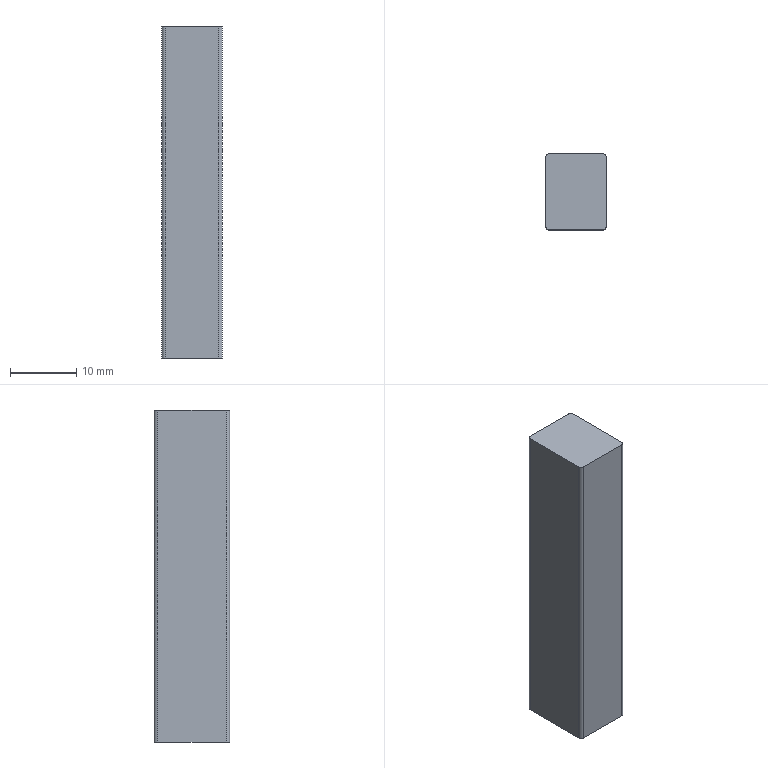Part | NX | features BREP 1 | 1 solid | 10 faces | box 9.124 x 11.391 x 50 mm | volume 5186 mm3 | plane 6 | cylinder 4 | commonest cylinder face diameters 1 x4
STEP:
#1=CARTESIAN_POINT('',(-4.062,5.695,-40.6));
#2=VERTEX_POINT('',#1);
#3=CARTESIAN_POINT('',(-4.562,5.195,-40.6));
#4=VERTEX_POINT('',#3);
#5=CARTESIAN_POINT('',(-4.062,5.195,-40.6));
#6=DIRECTION('',(0.,0.,1.));
#7=DIRECTION('',(1.,0.,0.));
#8=AXIS2_PLACEMENT_3D('',#5,#6,#7);
#9=CIRCLE('',#8,0.5);
#10=EDGE_CURVE('',#2,#4,#9,.T.);
#11=ORIENTED_EDGE('',*,*,#10,.F.);
#12=CARTESIAN_POINT('',(-4.062,5.695,-90.6));
#13=VERTEX_POINT('',#12);
#14=CARTESIAN_POINT('',(-4.062,5.695,-90.6));
#15=DIRECTION('',(0.,0.,1.));
#16=VECTOR('',#15,1000.);
#17=LINE('',#14,#16);
#18=EDGE_CURVE('',#13,#2,#17,.T.);
#19=ORIENTED_EDGE('',*,*,#18,.F.);
#20=CARTESIAN_POINT('',(-4.562,5.195,-90.6));
#21=VERTEX_POINT('',#20);
#22=CARTESIAN_POINT('',(-4.062,5.195,-90.6));
#23=DIRECTION('',(0.,0.,1.));
#24=DIRECTION('',(1.,0.,0.));
#25=AXIS2_PLACEMENT_3D('',#22,#23,#24);
#26=CIRCLE('',#25,0.5);
#27=EDGE_CURVE('',#13,#21,#26,.T.);
#28=ORIENTED_EDGE('',*,*,#27,.T.);
#29=CARTESIAN_POINT('',(-4.562,5.195,-90.6));
#30=DIRECTION('',(0.,0.,1.));
#31=VECTOR('',#30,1000.);
#32=LINE('',#29,#31);
#33=EDGE_CURVE('',#21,#4,#32,.T.);
#34=ORIENTED_EDGE('',*,*,#33,.T.);
#35=EDGE_LOOP('',(#11,#19,#28,#34));
#36=FACE_BOUND('',#35,.T.);
#37=CARTESIAN_POINT('',(-4.062,5.195,-90.6));
#38=DIRECTION('',(0.,0.,1.));
#39=DIRECTION('',(-1.,0.,0.));
#40=AXIS2_PLACEMENT_3D('',#37,#38,#39);
#41=CYLINDRICAL_SURFACE('',#40,0.5);
#42=ADVANCED_FACE('',(#36),#41,.T.);
#43=CARTESIAN_POINT('',(-4.562,-5.195,-40.6));
#44=VERTEX_POINT('',#43);
#45=CARTESIAN_POINT('',(-4.562,-5.195,-40.6));
#46=DIRECTION('',(0.,1.,0.));
#47=VECTOR('',#46,1000.);
#48=LINE('',#45,#47);
#49=EDGE_CURVE('',#44,#4,#48,.T.);
#50=ORIENTED_EDGE('',*,*,#49,.T.);
#51=ORIENTED_EDGE('',*,*,#33,.F.);
#52=CARTESIAN_POINT('',(-4.562,-5.195,-90.6));
#53=VERTEX_POINT('',#52);
#54=CARTESIAN_POINT('',(-4.562,-5.195,-90.6));
#55=DIRECTION('',(0.,1.,0.));
#56=VECTOR('',#55,1000.);
#57=LINE('',#54,#56);
#58=EDGE_CURVE('',#53,#21,#57,.T.);
#59=ORIENTED_EDGE('',*,*,#58,.F.);
#60=CARTESIAN_POINT('',(-4.562,-5.195,-90.6));
#61=DIRECTION('',(0.,0.,1.));
#62=VECTOR('',#61,1000.);
#63=LINE('',#60,#62);
#64=EDGE_CURVE('',#53,#44,#63,.T.);
#65=ORIENTED_EDGE('',*,*,#64,.T.);
#66=EDGE_LOOP('',(#50,#51,#59,#65));
#67=FACE_BOUND('',#66,.T.);
#68=CARTESIAN_POINT('',(-4.562,-5.195,-90.6));
#69=DIRECTION('',(1.,0.,0.));
#70=DIRECTION('',(0.,-1.,0.));
#71=AXIS2_PLACEMENT_3D('',#68,#69,#70);
#72=PLANE('',#71);
#73=ADVANCED_FACE('',(#67),#72,.F.);
#74=CARTESIAN_POINT('',(-4.062,-5.695,-40.6));
#75=VERTEX_POINT('',#74);
#76=CARTESIAN_POINT('',(-4.062,-5.195,-40.6));
#77=DIRECTION('',(0.,0.,1.));
#78=DIRECTION('',(1.,0.,0.));
#79=AXIS2_PLACEMENT_3D('',#76,#77,#78);
#80=CIRCLE('',#79,0.5);
#81=EDGE_CURVE('',#44,#75,#80,.T.);
#82=ORIENTED_EDGE('',*,*,#81,.F.);
#83=ORIENTED_EDGE('',*,*,#64,.F.);
#84=CARTESIAN_POINT('',(-4.062,-5.695,-90.6));
#85=VERTEX_POINT('',#84);
#86=CARTESIAN_POINT('',(-4.062,-5.195,-90.6));
#87=DIRECTION('',(0.,0.,1.));
#88=DIRECTION('',(1.,0.,0.));
#89=AXIS2_PLACEMENT_3D('',#86,#87,#88);
#90=CIRCLE('',#89,0.5);
#91=EDGE_CURVE('',#53,#85,#90,.T.);
#92=ORIENTED_EDGE('',*,*,#91,.T.);
#93=CARTESIAN_POINT('',(-4.062,-5.695,-90.6));
#94=DIRECTION('',(0.,0.,1.));
#95=VECTOR('',#94,1000.);
#96=LINE('',#93,#95);
#97=EDGE_CURVE('',#85,#75,#96,.T.);
#98=ORIENTED_EDGE('',*,*,#97,.T.);
#99=EDGE_LOOP('',(#82,#83,#92,#98));
#100=FACE_BOUND('',#99,.T.);
#101=CARTESIAN_POINT('',(-4.062,-5.195,-90.6));
#102=DIRECTION('',(0.,0.,1.));
#103=DIRECTION('',(-1.,0.,0.));
#104=AXIS2_PLACEMENT_3D('',#101,#102,#103);
#105=CYLINDRICAL_SURFACE('',#104,0.5);
#106=ADVANCED_FACE('',(#100),#105,.T.);
#107=CARTESIAN_POINT('',(4.062,-5.695,-40.6));
#108=VERTEX_POINT('',#107);
#109=CARTESIAN_POINT('',(4.062,-5.695,-40.6));
#110=DIRECTION('',(-1.,0.,0.));
#111=VECTOR('',#110,1000.);
#112=LINE('',#109,#111);
#113=EDGE_CURVE('',#108,#75,#112,.T.);
#114=ORIENTED_EDGE('',*,*,#113,.T.);
#115=ORIENTED_EDGE('',*,*,#97,.F.);
#116=CARTESIAN_POINT('',(4.062,-5.695,-90.6));
#117=VERTEX_POINT('',#116);
#118=CARTESIAN_POINT('',(4.062,-5.695,-90.6));
#119=DIRECTION('',(-1.,0.,0.));
#120=VECTOR('',#119,1000.);
#121=LINE('',#118,#120);
#122=EDGE_CURVE('',#117,#85,#121,.T.);
#123=ORIENTED_EDGE('',*,*,#122,.F.);
#124=CARTESIAN_POINT('',(4.062,-5.695,-90.6));
#125=DIRECTION('',(0.,0.,1.));
#126=VECTOR('',#125,1000.);
#127=LINE('',#124,#126);
#128=EDGE_CURVE('',#117,#108,#127,.T.);
#129=ORIENTED_EDGE('',*,*,#128,.T.);
#130=EDGE_LOOP('',(#114,#115,#123,#129));
#131=FACE_BOUND('',#130,.T.);
#132=CARTESIAN_POINT('',(4.062,-5.695,-90.6));
#133=DIRECTION('',(0.,1.,0.));
#134=DIRECTION('',(0.,0.,-1.));
#135=AXIS2_PLACEMENT_3D('',#132,#133,#134);
#136=PLANE('',#135);
#137=ADVANCED_FACE('',(#131),#136,.F.);
#138=CARTESIAN_POINT('',(4.562,-5.195,-40.6));
#139=VERTEX_POINT('',#138);
#140=CARTESIAN_POINT('',(4.062,-5.195,-40.6));
#141=DIRECTION('',(0.,0.,1.));
#142=DIRECTION('',(1.,0.,0.));
#143=AXIS2_PLACEMENT_3D('',#140,#141,#142);
#144=CIRCLE('',#143,0.5);
#145=EDGE_CURVE('',#108,#139,#144,.T.);
#146=ORIENTED_EDGE('',*,*,#145,.F.);
#147=ORIENTED_EDGE('',*,*,#128,.F.);
#148=CARTESIAN_POINT('',(4.562,-5.195,-90.6));
#149=VERTEX_POINT('',#148);
#150=CARTESIAN_POINT('',(4.062,-5.195,-90.6));
#151=DIRECTION('',(0.,0.,1.));
#152=DIRECTION('',(1.,0.,0.));
#153=AXIS2_PLACEMENT_3D('',#150,#151,#152);
#154=CIRCLE('',#153,0.5);
#155=EDGE_CURVE('',#117,#149,#154,.T.);
#156=ORIENTED_EDGE('',*,*,#155,.T.);
#157=CARTESIAN_POINT('',(4.562,-5.195,-90.6));
#158=DIRECTION('',(0.,0.,1.));
#159=VECTOR('',#158,1000.);
#160=LINE('',#157,#159);
#161=EDGE_CURVE('',#149,#139,#160,.T.);
#162=ORIENTED_EDGE('',*,*,#161,.T.);
#163=EDGE_LOOP('',(#146,#147,#156,#162));
#164=FACE_BOUND('',#163,.T.);
#165=CARTESIAN_POINT('',(4.062,-5.195,-90.6));
#166=DIRECTION('',(0.,0.,1.));
#167=DIRECTION('',(-1.,0.,0.));
#168=AXIS2_PLACEMENT_3D('',#165,#166,#167);
#169=CYLINDRICAL_SURFACE('',#168,0.5);
#170=ADVANCED_FACE('',(#164),#169,.T.);
#171=CARTESIAN_POINT('',(4.562,5.195,-40.6));
#172=VERTEX_POINT('',#171);
#173=CARTESIAN_POINT('',(4.562,5.195,-40.6));
#174=DIRECTION('',(0.,-1.,0.));
#175=VECTOR('',#174,1000.);
#176=LINE('',#173,#175);
#177=EDGE_CURVE('',#172,#139,#176,.T.);
#178=ORIENTED_EDGE('',*,*,#177,.T.);
#179=ORIENTED_EDGE('',*,*,#161,.F.);
#180=CARTESIAN_POINT('',(4.562,5.195,-90.6));
#181=VERTEX_POINT('',#180);
#182=CARTESIAN_POINT('',(4.562,5.195,-90.6));
#183=DIRECTION('',(0.,-1.,0.));
#184=VECTOR('',#183,1000.);
#185=LINE('',#182,#184);
#186=EDGE_CURVE('',#181,#149,#185,.T.);
#187=ORIENTED_EDGE('',*,*,#186,.F.);
#188=CARTESIAN_POINT('',(4.562,5.195,-90.6));
#189=DIRECTION('',(0.,0.,1.));
#190=VECTOR('',#189,1000.);
#191=LINE('',#188,#190);
#192=EDGE_CURVE('',#181,#172,#191,.T.);
#193=ORIENTED_EDGE('',*,*,#192,.T.);
#194=EDGE_LOOP('',(#178,#179,#187,#193));
#195=FACE_BOUND('',#194,.T.);
#196=CARTESIAN_POINT('',(4.562,5.195,-90.6));
#197=DIRECTION('',(-1.,0.,0.));
#198=DIRECTION('',(0.,0.,-1.));
#199=AXIS2_PLACEMENT_3D('',#196,#197,#198);
#200=PLANE('',#199);
#201=ADVANCED_FACE('',(#195),#200,.F.);
#202=CARTESIAN_POINT('',(4.062,5.695,-40.6));
#203=VERTEX_POINT('',#202);
#204=CARTESIAN_POINT('',(4.062,5.195,-40.6));
#205=DIRECTION('',(0.,0.,1.));
#206=DIRECTION('',(1.,0.,0.));
#207=AXIS2_PLACEMENT_3D('',#204,#205,#206);
#208=CIRCLE('',#207,0.5);
#209=EDGE_CURVE('',#172,#203,#208,.T.);
#210=ORIENTED_EDGE('',*,*,#209,.F.);
#211=ORIENTED_EDGE('',*,*,#192,.F.);
#212=CARTESIAN_POINT('',(4.062,5.695,-90.6));
#213=VERTEX_POINT('',#212);
#214=CARTESIAN_POINT('',(4.062,5.195,-90.6));
#215=DIRECTION('',(0.,0.,1.));
#216=DIRECTION('',(1.,0.,0.));
#217=AXIS2_PLACEMENT_3D('',#214,#215,#216);
#218=CIRCLE('',#217,0.5);
#219=EDGE_CURVE('',#181,#213,#218,.T.);
#220=ORIENTED_EDGE('',*,*,#219,.T.);
#221=CARTESIAN_POINT('',(4.062,5.695,-90.6));
#222=DIRECTION('',(0.,0.,1.));
#223=VECTOR('',#222,1000.);
#224=LINE('',#221,#223);
#225=EDGE_CURVE('',#213,#203,#224,.T.);
#226=ORIENTED_EDGE('',*,*,#225,.T.);
#227=EDGE_LOOP('',(#210,#211,#220,#226));
#228=FACE_BOUND('',#227,.T.);
#229=CARTESIAN_POINT('',(4.062,5.195,-90.6));
#230=DIRECTION('',(0.,0.,1.));
#231=DIRECTION('',(-1.,0.,0.));
#232=AXIS2_PLACEMENT_3D('',#229,#230,#231);
#233=CYLINDRICAL_SURFACE('',#232,0.5);
#234=ADVANCED_FACE('',(#228),#233,.T.);
#235=CARTESIAN_POINT('',(-4.062,5.695,-40.6));
#236=DIRECTION('',(1.,0.,0.));
#237=VECTOR('',#236,1000.);
#238=LINE('',#235,#237);
#239=EDGE_CURVE('',#2,#203,#238,.T.);
#240=ORIENTED_EDGE('',*,*,#239,.T.);
#241=ORIENTED_EDGE('',*,*,#225,.F.);
#242=CARTESIAN_POINT('',(-4.062,5.695,-90.6));
#243=DIRECTION('',(1.,0.,0.));
#244=VECTOR('',#243,1000.);
#245=LINE('',#242,#244);
#246=EDGE_CURVE('',#13,#213,#245,.T.);
#247=ORIENTED_EDGE('',*,*,#246,.F.);
#248=ORIENTED_EDGE('',*,*,#18,.T.);
#249=EDGE_LOOP('',(#240,#241,#247,#248));
#250=FACE_BOUND('',#249,.T.);
#251=CARTESIAN_POINT('',(-4.062,5.695,-90.6));
#252=DIRECTION('',(0.,-1.,0.));
#253=DIRECTION('',(0.,0.,1.));
#254=AXIS2_PLACEMENT_3D('',#251,#252,#253);
#255=PLANE('',#254);
#256=ADVANCED_FACE('',(#250),#255,.F.);
#257=ORIENTED_EDGE('',*,*,#27,.F.);
#258=ORIENTED_EDGE('',*,*,#246,.T.);
#259=ORIENTED_EDGE('',*,*,#219,.F.);
#260=ORIENTED_EDGE('',*,*,#186,.T.);
#261=ORIENTED_EDGE('',*,*,#155,.F.);
#262=ORIENTED_EDGE('',*,*,#122,.T.);
#263=ORIENTED_EDGE('',*,*,#91,.F.);
#264=ORIENTED_EDGE('',*,*,#58,.T.);
#265=EDGE_LOOP('',(#257,#258,#259,#260,#261,#262,#263,#264));
#266=FACE_BOUND('',#265,.T.);
#267=CARTESIAN_POINT('',(-4.062,5.195,-90.6));
#268=DIRECTION('',(0.,0.,1.));
#269=DIRECTION('',(-1.,0.,0.));
#270=AXIS2_PLACEMENT_3D('',#267,#268,#269);
#271=PLANE('',#270);
#272=ADVANCED_FACE('',(#266),#271,.F.);
#273=ORIENTED_EDGE('',*,*,#10,.T.);
#274=ORIENTED_EDGE('',*,*,#49,.F.);
#275=ORIENTED_EDGE('',*,*,#81,.T.);
#276=ORIENTED_EDGE('',*,*,#113,.F.);
#277=ORIENTED_EDGE('',*,*,#145,.T.);
#278=ORIENTED_EDGE('',*,*,#177,.F.);
#279=ORIENTED_EDGE('',*,*,#209,.T.);
#280=ORIENTED_EDGE('',*,*,#239,.F.);
#281=EDGE_LOOP('',(#273,#274,#275,#276,#277,#278,#279,#280));
#282=FACE_BOUND('',#281,.T.);
#283=CARTESIAN_POINT('',(-4.062,5.195,-40.6));
#284=DIRECTION('',(0.,0.,1.));
#285=DIRECTION('',(-1.,0.,0.));
#286=AXIS2_PLACEMENT_3D('',#283,#284,#285);
#287=PLANE('',#286);
#288=ADVANCED_FACE('',(#282),#287,.T.);
#289=CLOSED_SHELL('',(#42,#73,#106,#137,#170,#201,#234,#256,#272,#288));
#290=MANIFOLD_SOLID_BREP('',#289);
#291=(LENGTH_UNIT()NAMED_UNIT(*)SI_UNIT(.MILLI.,.METRE.));
#292=UNCERTAINTY_MEASURE_WITH_UNIT(LENGTH_MEASURE(0.00001),#291,'','');
#293=(NAMED_UNIT(*)PLANE_ANGLE_UNIT()SI_UNIT($,.RADIAN.));
#294=(NAMED_UNIT(*)SI_UNIT($,.STERADIAN.)SOLID_ANGLE_UNIT());
#295=(GEOMETRIC_REPRESENTATION_CONTEXT(3)GLOBAL_UNCERTAINTY_ASSIGNED_CONTEXT((#292))GLOBAL_UNIT_ASSIGNED_CONTEXT((#291,#293,#294))REPRESENTATION_CONTEXT('',''));
#296=ADVANCED_BREP_SHAPE_REPRESENTATION('',(#290),#295);